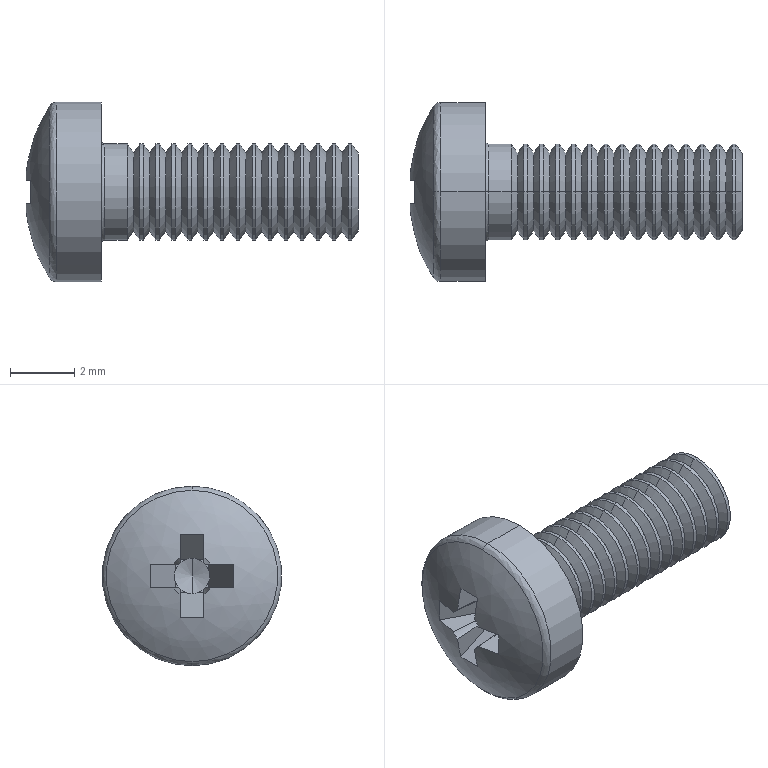Part | SolidWorks | features BaseBody 1 | 1 solid | 128 faces | box 10.354 x 5.6 x 5.6 mm | volume 94.439 mm3 | cone 69 | cylinder 32 | plane 22 | spline 5 | commonest cylinder face diameters 3 x30 5.6 x2